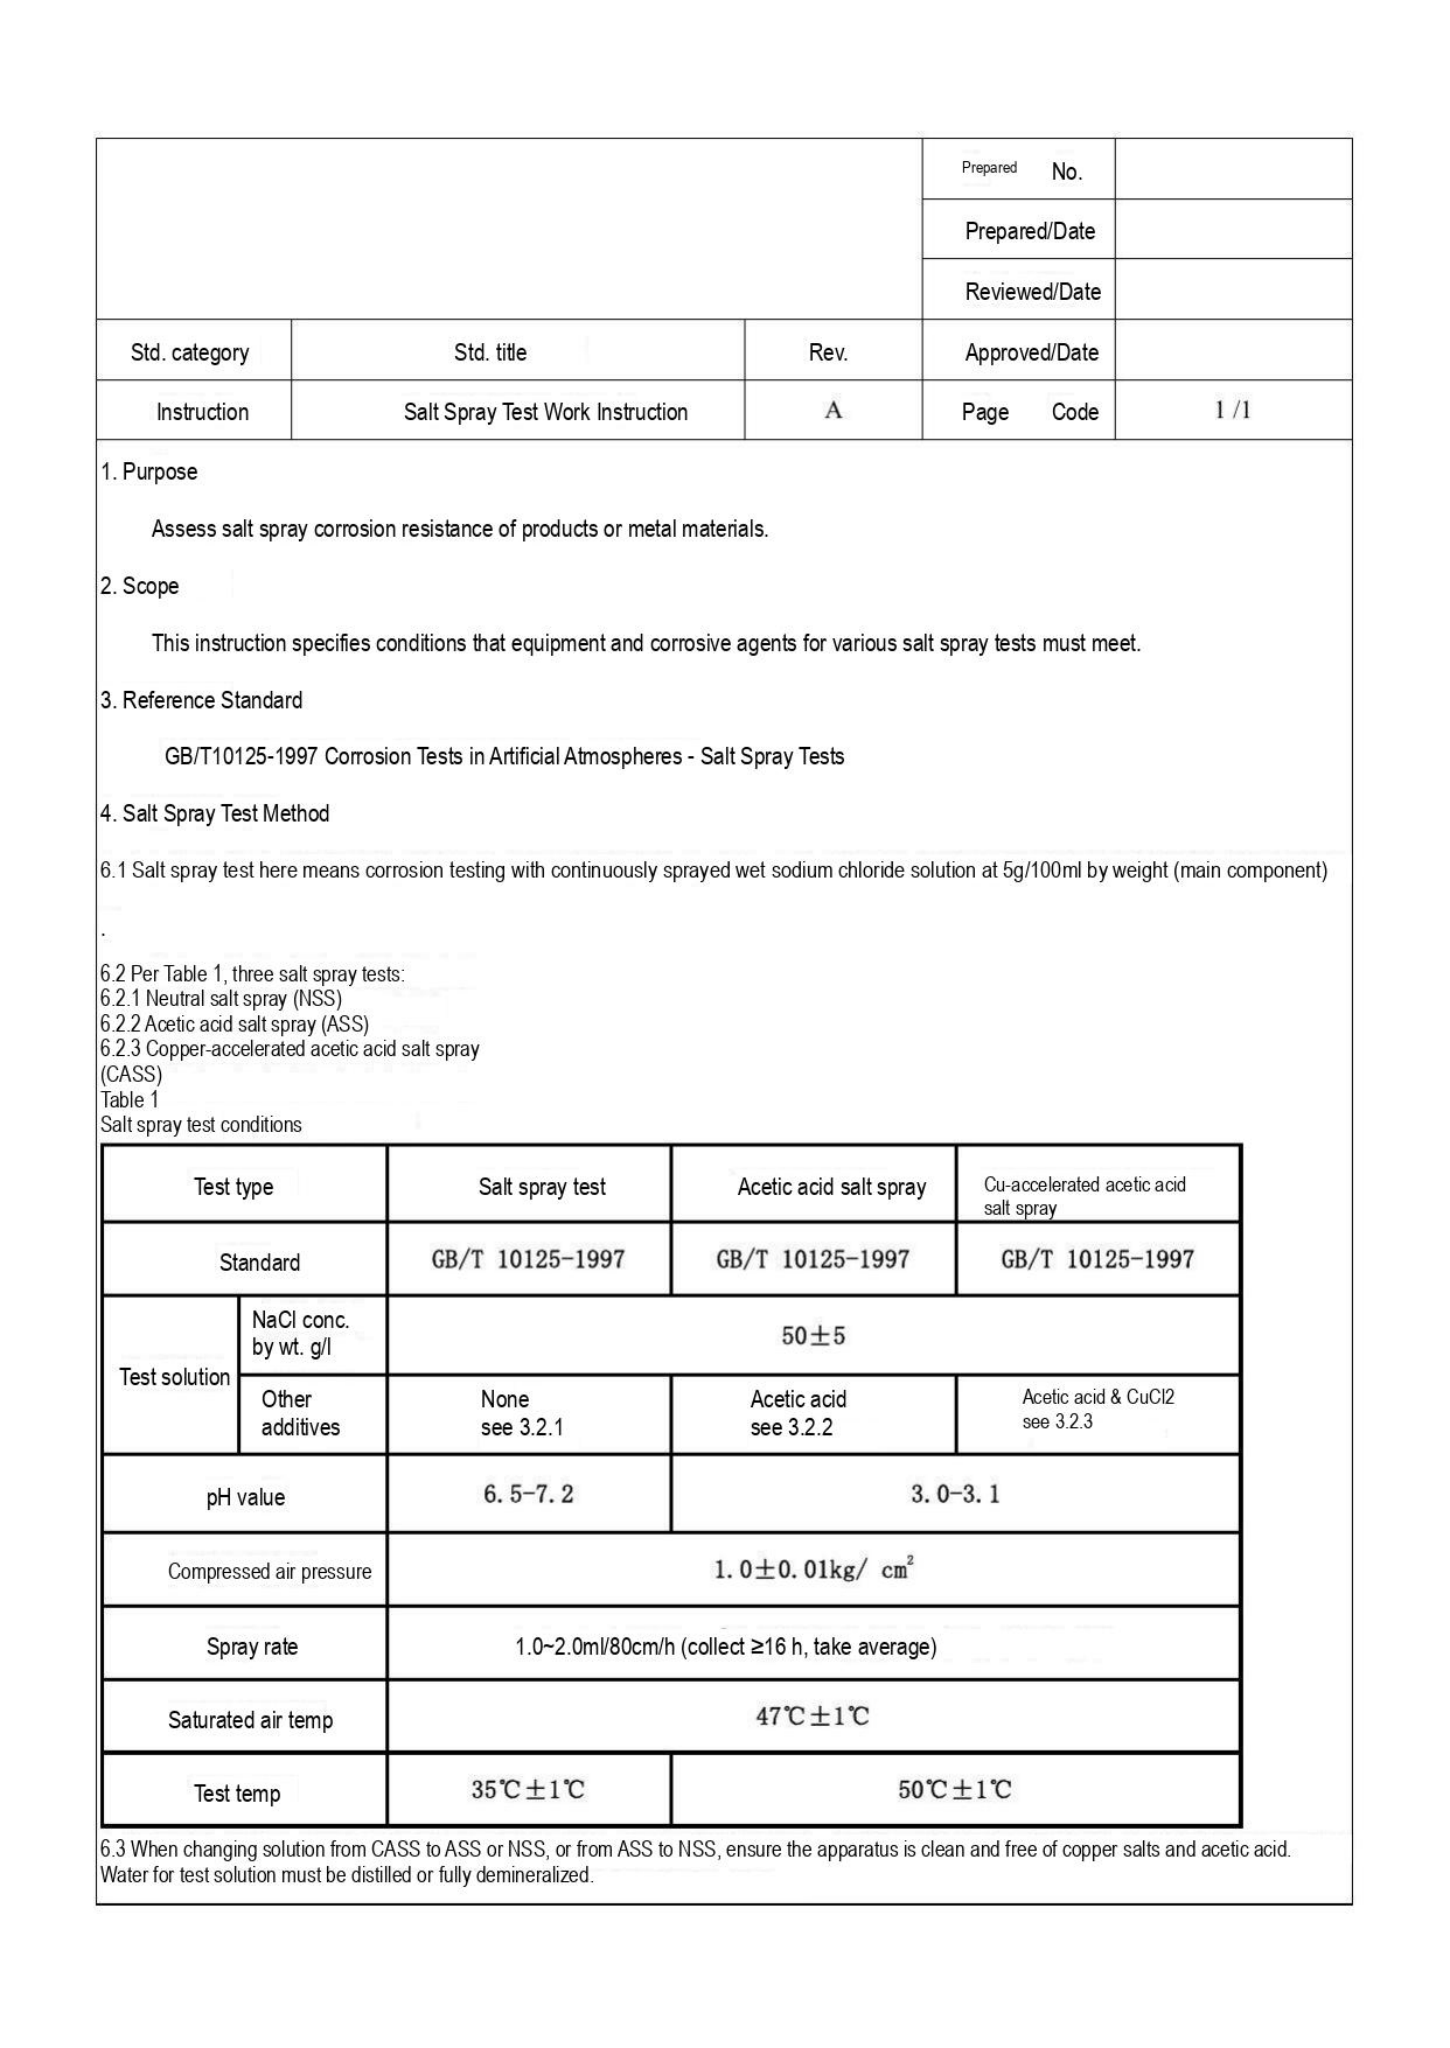| | | | Prepared No. | |
|---|---|---|---|---|
| | | | Prepared/Date | |
| | | | Reviewed/Date | |
| Std. category | Std. title | Rev. | Approved/Date | |
| Instruction | Salt Spray Test Work Instruction | A | Page Code | 1 /1 |

1. Purpose

Assess salt spray corrosion resistance of products or metal materials.

2. Scope

This instruction specifies conditions that equipment and corrosive agents for various salt spray tests must meet.

3. Reference Standard

GB/T10125-1997 Corrosion Tests in Artificial Atmospheres - Salt Spray Tests

4. Salt Spray Test Method

6.1 Salt spray test here means corrosion testing with continuously sprayed wet sodium chloride solution at 5g/100ml by weight (main component)

.

6.2 Per Table 1, three salt spray tests:
6.2.1 Neutral salt spray (NSS)
6.2.2 Acetic acid salt spray (ASS)
6.2.3 Copper-accelerated acetic acid salt spray (CASS)
Table 1
Salt spray test conditions

| Test type | | Salt spray test | Acetic acid salt spray | Cu-accelerated acetic acid salt spray |
|---|---|---|---|---|
| Standard | | GB/T 10125-1997 | GB/T 10125-1997 | GB/T 10125-1997 |
| Test solution | NaCl conc. by wt. g/l | 50±5 | | |
| | Other additives | None see 3.2.1 | Acetic acid see 3.2.2 | Acetic acid & CuCl2 see 3.2.3 |
| pH value | | 6. 5-7. 2 | 3. 0-3. 1 | |
| Compressed air pressure | | 1. 0±0. 01kg/ cm² | | |
| Spray rate | | 1.0~2.0ml/80cm/h (collect ≥16 h, take average) | | |
| Saturated air temp | | 47℃±1℃ | | |
| Test temp | | 35℃±1℃ | 50℃±1℃ | |

6.3 When changing solution from CASS to ASS or NSS, or from ASS to NSS, ensure the apparatus is clean and free of copper salts and acetic acid. Water for test solution must be distilled or fully demineralized.
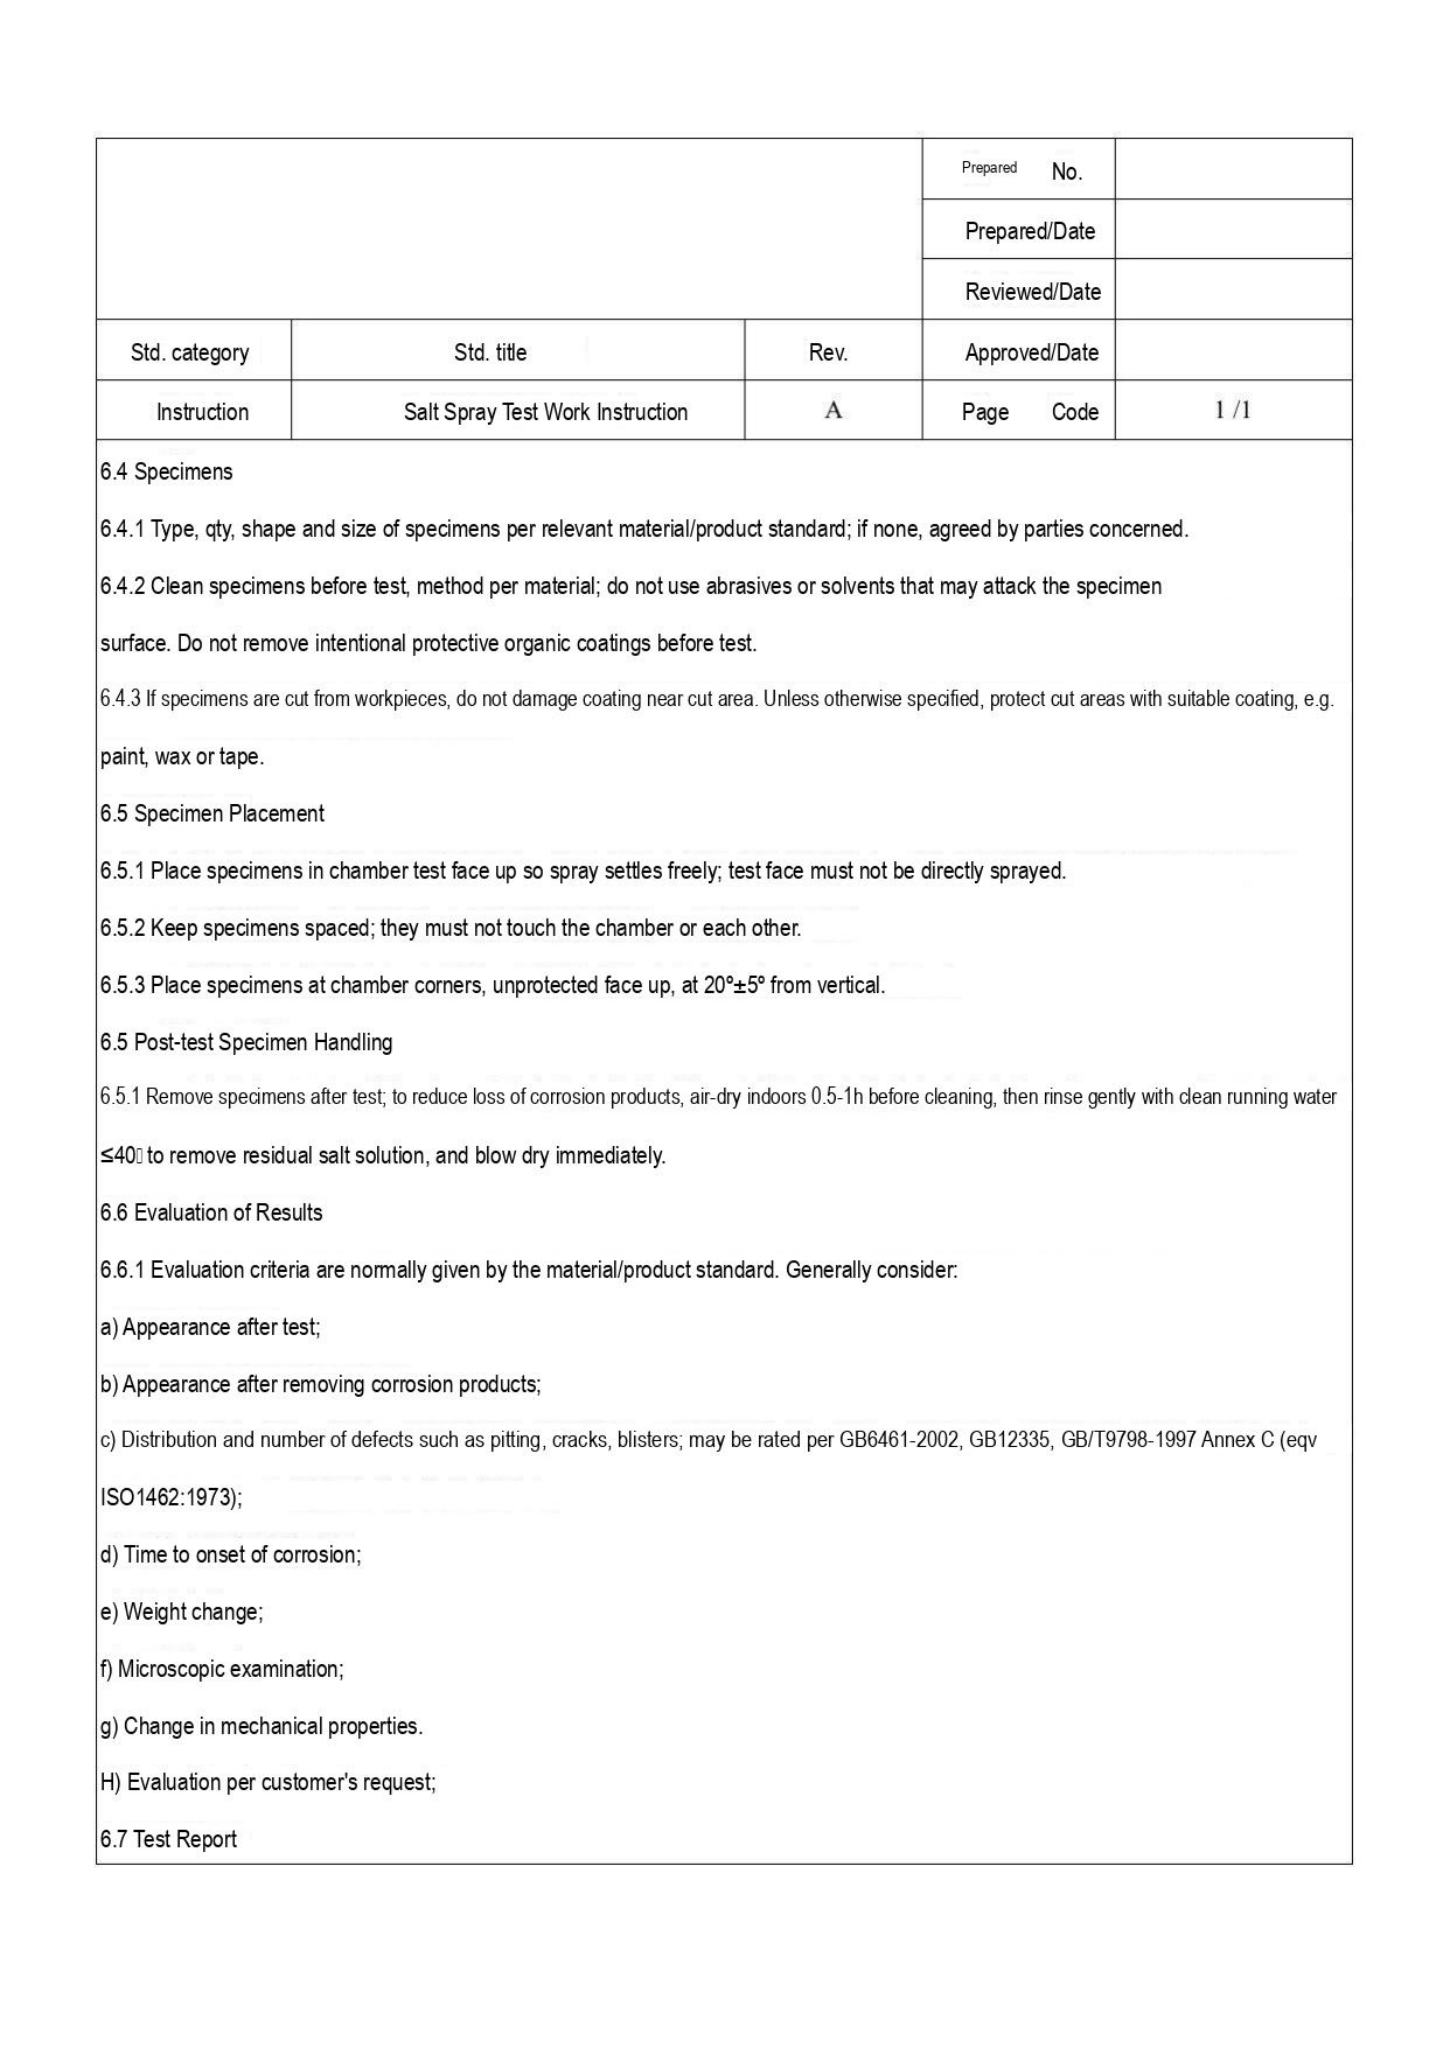| | | | Prepared No. | |
|---|---|---|---|---|
| | | | Prepared/Date | |
| | | | Reviewed/Date | |
| Std. category | Std. title | Rev. | Approved/Date | |
| Instruction | Salt Spray Test Work Instruction | A | Page Code | 1 /1 |

6.4 Specimens

6.4.1 Type, qty, shape and size of specimens per relevant material/product standard; if none, agreed by parties concerned.

6.4.2 Clean specimens before test, method per material; do not use abrasives or solvents that may attack the specimen surface. Do not remove intentional protective organic coatings before test.

6.4.3 If specimens are cut from workpieces, do not damage coating near cut area. Unless otherwise specified, protect cut areas with suitable coating, e.g. paint, wax or tape.

6.5 Specimen Placement

6.5.1 Place specimens in chamber test face up so spray settles freely; test face must not be directly sprayed.

6.5.2 Keep specimens spaced; they must not touch the chamber or each other.

6.5.3 Place specimens at chamber corners, unprotected face up, at 20°±5° from vertical.

6.5 Post-test Specimen Handling

6.5.1 Remove specimens after test; to reduce loss of corrosion products, air-dry indoors 0.5-1h before cleaning, then rinse gently with clean running water ≤40 to remove residual salt solution, and blow dry immediately.

6.6 Evaluation of Results

6.6.1 Evaluation criteria are normally given by the material/product standard. Generally consider:

a) Appearance after test;

b) Appearance after removing corrosion products;

c) Distribution and number of defects such as pitting, cracks, blisters; may be rated per GB6461-2002, GB12335, GB/T9798-1997 Annex C (eqv ISO1462:1973);

d) Time to onset of corrosion;

e) Weight change;

f) Microscopic examination;

g) Change in mechanical properties.

H) Evaluation per customer's request;

6.7 Test Report
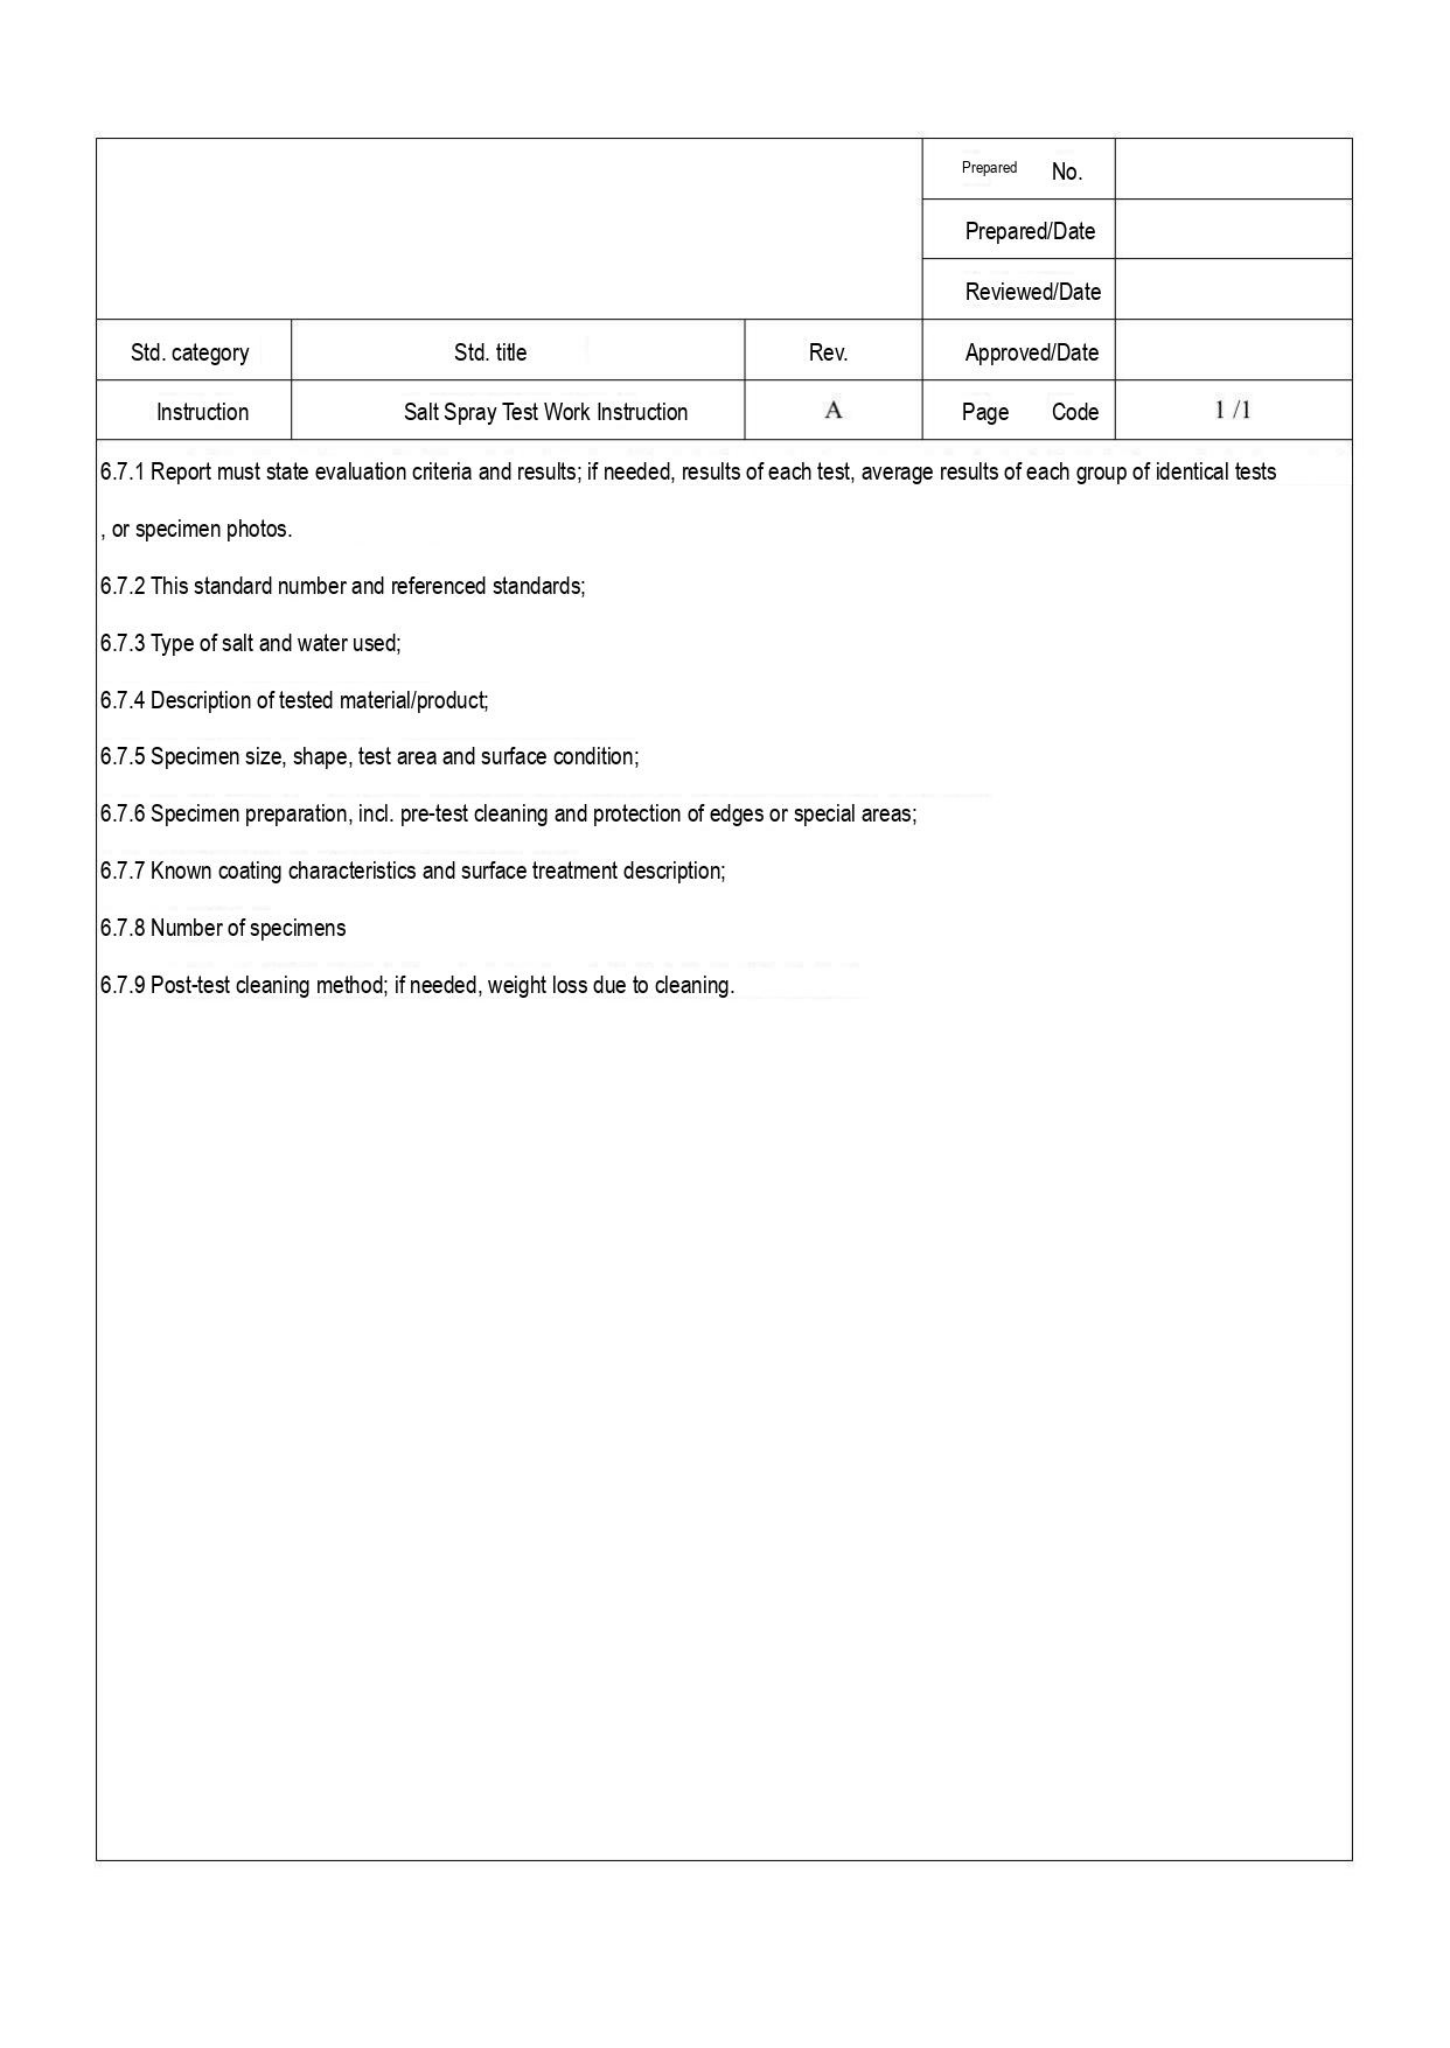| | | | Prepared No. | |
|---|---|---|---|---|
| | | | Prepared/Date | |
| | | | Reviewed/Date | |
| Std. category | Std. title | Rev. | Approved/Date | |
| Instruction | Salt Spray Test Work Instruction | A | Page Code | 1 /1 |

6.7.1 Report must state evaluation criteria and results; if needed, results of each test, average results of each group of identical tests, or specimen photos.

6.7.2 This standard number and referenced standards;

6.7.3 Type of salt and water used;

6.7.4 Description of tested material/product;

6.7.5 Specimen size, shape, test area and surface condition;

6.7.6 Specimen preparation, incl. pre-test cleaning and protection of edges or special areas;

6.7.7 Known coating characteristics and surface treatment description;

6.7.8 Number of specimens

6.7.9 Post-test cleaning method; if needed, weight loss due to cleaning.